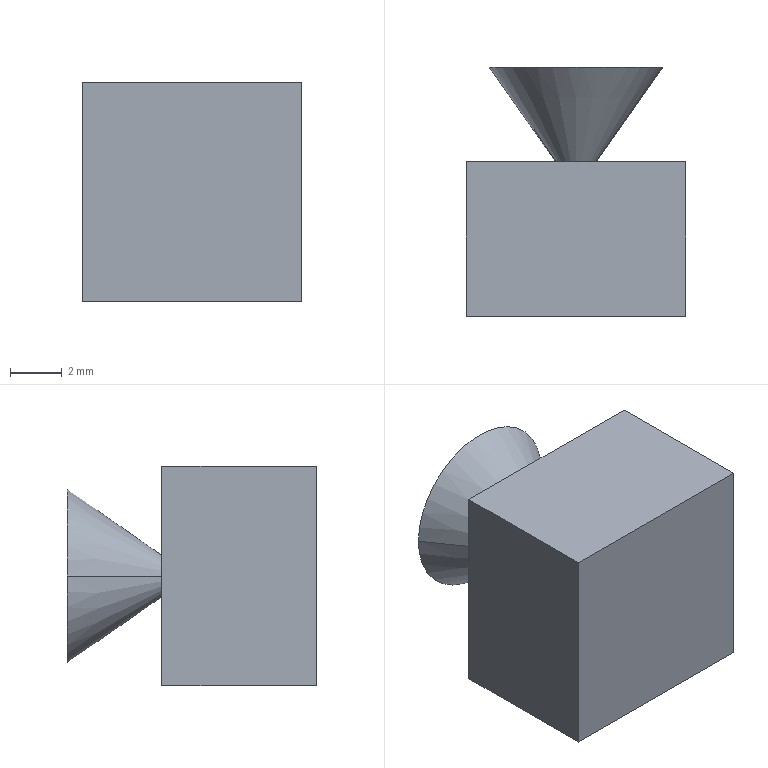Part | Creo | 1 solid | 14 faces | box 8.5 x 9.659 x 8.5 mm | volume 422.481 mm3 | plane 8 | cylinder 4 | cone 2 | commonest cylinder face diameters 5.5 x2 6.5 x2